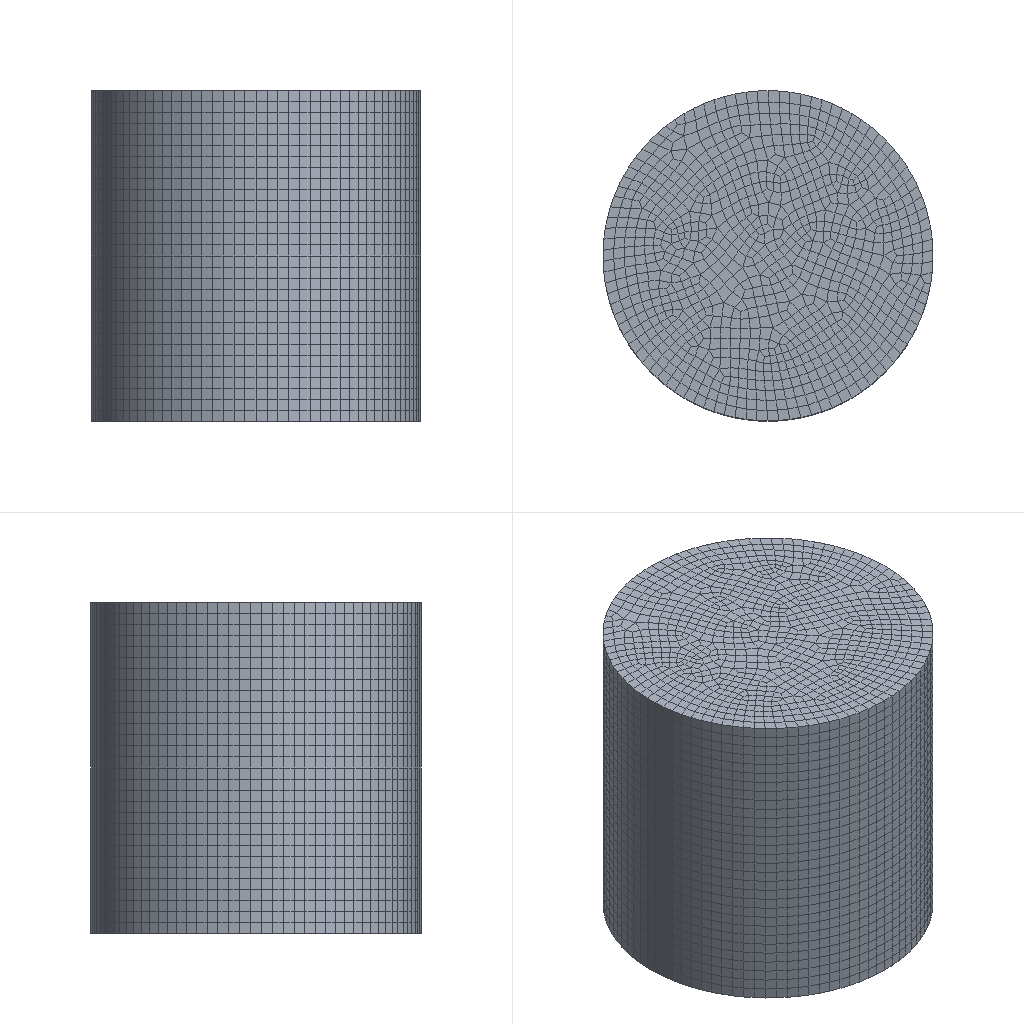Simulation study | abaqus
Set-up summary:
category,name,step,type,value,unit,region
solver,abaqus
solver,version,,,Abaqus/Explicit 2020
units,not stated in the deck,,not stated
analysis,deck,,transient,transient
load_step,Step-1,Step-1,transient,nlgeom=True
contact,interactions,,,general=0 pairs=2 ties=0
load_step,requested,,,1
mesh,nodes,,,72803
mesh,elements,,,70558
element_type,R3D3,,rigid,384
element_type,R3D4,,rigid,41884
element_type,C3D8R,,solid,28290
load,load commands in deck,,count,1
bc,support commands in deck,,count,4
material,MG,,in results
material,TC,,in results
check,setup vs results,,match,"per instance, exact: element labels, types and connectivity; labels of the nodes the elements use; coordinates of those nodes at SINGLE_PRECISION in 3 of 3 instance(s)"
Abaqus input file, long lists of numbers shortened:
*Heading
** Job name: Job-1 Model name: Model-1
** Generated by: Abaqus/CAE 2020
*Preprint, echo=NO, model=NO, history=NO, contact=NO
**
** PARTS
**
*Part, name=gan
*Node
      1,           0.,         -9.5,          20.
      2,           0.,         -9.5,           0.
** (21038 more lines like these left out)
*Element, type=R3D4
    1,     1,     3,   399,   597
    2,     3,     4,   400,   399
** (20940 more lines like these left out)
*Element, type=R3D3
13334, 16695, 14745, 14780
13335, 16883, 14935, 14929
** (190 more lines like these left out)
*Node
  21041,           0., -5.81707235e-16,          20.
*Nset, nset=gan-RefPt_, internal
21041,
*Elset, elset=gan, generate
     1,  21134,      1
*End Part
**
*Part, name=work
*Node
      1,  0.5976,  -2.94,           0.
      2,   1.353,  -2.678,           0.
** (30719 more lines like these left out)
*Element, type=C3D8R
    1,  1085,  1134,  1197,  1018,    94,   143,   206,    27
    2,  1170,  1022,  1021,  1183,   179,    31,    30,   192
** (28288 more lines like these left out)
*Nset, nset=Set-1, generate
     1,  30721,      1
*Elset, elset=Set-1, generate
     1,  28290,      1
** Section: mg
*Solid Section, elset=Set-1, material=mg
,
*End Part
**
**
** ASSEMBLY
**
*Assembly, name=Assembly
**
*Instance, name=work-1, part=work
          0.,           0.,          -6.
*End Instance
**
*Instance, name=gan-1, part=gan
*End Instance
**
*Instance, name=gan-1-lin-2-1, part=gan
          0.,           0.,         -26.
*End Instance
**
*Nset, nset=Set-1, instance=gan-1-lin-2-1
 21041,
*Nset, nset=Set-2, instance=gan-1
 21041,
*Nset, nset=Set-3, instance=gan-1
 21041,
*Nset, nset=Set-4, instance=gan-1
 21041,
*Elset, elset=_m_Surf-1_SPOS, internal, instance=gan-1, generate
 17221,  21134,      1
*Surface, type=ELEMENT, name=m_Surf-1
_m_Surf-1_SPOS, SPOS
*Elset, elset=_m_Surf-3_SPOS, internal, instance=gan-1-lin-2-1, generate
 13334,  17220,      1
*Surface, type=ELEMENT, name=m_Surf-3
_m_Surf-3_SPOS, SPOS
*Elset, elset=_s_Surf-1_S1, internal, instance=work-1, generate
 27348,  28290,      1
*Surface, type=ELEMENT, name=s_Surf-1
_s_Surf-1_S1, S1
*Elset, elset=_s_Surf-3_S2, internal, instance=work-1, generate
   1,  943,    1
*Surface, type=ELEMENT, name=s_Surf-3
_s_Surf-3_S2, S2
*Rigid Body, ref node=gan-1.gan-RefPt_, elset=gan-1.gan
*Rigid Body, ref node=gan-1-lin-2-1.gan-RefPt_, elset=gan-1-lin-2-1.gan
*Element, type=MASS, elset=Set-4_Inertia-1_
1, gan-1.21
*Mass, elset=Set-4_Inertia-1_
0.001,
*End Assembly
*Amplitude, name=Amp-1
             0.,              0.,           0.125,              1.
**
** MATERIALS
**
*Material, name=mg
*Damage Initiation, criterion=DUCTILE
 0.15, 0.8,  0.
*Damage Evolution, type=DISPLACEMENT
 0.0001,
*Density
 2.67e-09,
*Elastic
45000., 0.3
*Plastic
165.,    0.
180., 0.002
250.,  0.05
280.,   0.1
*Material, name=tc
*Density
 4.5e-09,
*Elastic
184950., 0.2
**
** INTERACTION PROPERTIES
**
*Surface Interaction, name=IntProp-1
*Friction
 0.35,
*Surface Behavior, pressure-overclosure=HARD
**
** PREDEFINED FIELDS
**
** Name: Predefined Field-1   Type: Velocity
*Initial Conditions, type=VELOCITY
Set-3, 1, 0.
Set-3, 2, 0.
Set-3, 3, -8000.
** ----------------------------------------------------------------
**
** STEP: Step-1
**
*Step, name=Step-1, nlgeom=YES
*Dynamic, Explicit
, 0.0001
*Bulk Viscosity
0.06, 1.2
**
** BOUNDARY CONDITIONS
**
** Name: BC-1 Type: 对称/反对称/完全固定
*Boundary
Set-1, ENCASTRE
** Name: BC-2 Type: 位移/转角
*Boundary
Set-2, 4, 4
Set-2, 5, 5
Set-2, 6, 6
**
** INTERACTIONS
**
** Interaction: Int-1
*Contact Pair, interaction=IntProp-1, mechanical constraint=KINEMATIC, cpset=Int-1
m_Surf-1, s_Surf-1
** Interaction: Int-2
*Contact Pair, interaction=IntProp-1, mechanical constraint=KINEMATIC, cpset=Int-2
m_Surf-3, s_Surf-3
**
** OUTPUT REQUESTS
**
*Restart, write, number interval=1, time marks=NO
**
** FIELD OUTPUT: F-Output-1
**
*Output, field, number interval=50
*Node Output
A, CF, RF, RM, RT, U, V
*Element Output, directions=YES
E, EVF, LE, MISES, MISESMAX, MISESONLY, NE, PE, PEEQ, PEEQMAX, PEEQT, PEEQVAVG, PEMAG, PEVAVG, PRESSONLY, S
SEQUT, SF, SSAVG, STATUS, SVAVG, YIELDPOT
*Contact Output
CSTRESS,
**
** HISTORY OUTPUT: H-Output-1
**
*Output, history, variable=PRESELECT
*End Step
Results summary:
result,step,Step-1,completed,increments=4824 time=9.999999747378752e-05/9.999999747378752e-05
result,analysis,,,transient
result,last_loadstep,,,1
result,analysis steps,,count,1
result,primary field,,,U
result,reaction total,,FX,0.0,model units
result,reaction total,,FY,0.0,model units
result,reaction total,,FZ,0.0,model units